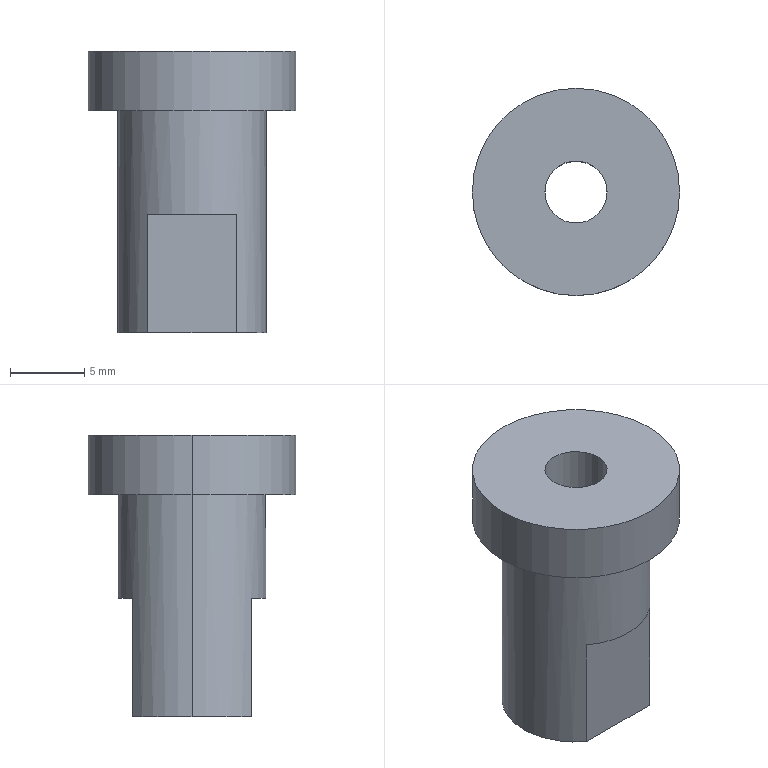Part | STEP file | PN_0015 Mount electronic clip cylinder connecting head | 1 solid | 13 faces | box 14 x 14 x 19 mm | volume 1465 mm3 | plane 7 | cylinder 6 | commonest cylinder face diameters 4.2 x2 10 x2 14 x2
STEP:
#1=CARTESIAN_POINT('',(0.,0.,0.));
#2=DIRECTION('',(0.,0.,1.));
#3=DIRECTION('',(1.,0.,0.));
#4=AXIS2_PLACEMENT_3D('',#1,#2,#3);
#5=CARTESIAN_POINT('',(-2.1,0.,19.));
#6=VERTEX_POINT('',#5);
#7=CARTESIAN_POINT('',(-2.1,0.,0.));
#8=VERTEX_POINT('',#7);
#9=CARTESIAN_POINT('',(-2.1,0.,0.));
#10=DIRECTION('',(0.,0.,-1.));
#11=VECTOR('',#10,1.);
#12=LINE('',#9,#11);
#13=CARTESIAN_POINT('',(0.,0.,0.));
#14=DIRECTION('',(0.,0.,-1.));
#15=DIRECTION('',(-1.,0.,0.));
#16=AXIS2_PLACEMENT_3D('',#13,#14,#15);
#17=CYLINDRICAL_SURFACE('',#16,2.1);
#18=CARTESIAN_POINT('',(6.283,0.));
#19=DIRECTION('',(0.,1.));
#20=VECTOR('',#19,1.);
#21=LINE('',#18,#20);
#22=(GEOMETRIC_REPRESENTATION_CONTEXT(2)PARAMETRIC_REPRESENTATION_CONTEXT()REPRESENTATION_CONTEXT('',''));
#23=DEFINITIONAL_REPRESENTATION('',(#21),#22);
#24=PCURVE('',#17,#23);
#25=CARTESIAN_POINT('',(0.,0.,0.));
#26=DIRECTION('',(0.,0.,-1.));
#27=DIRECTION('',(-1.,0.,0.));
#28=AXIS2_PLACEMENT_3D('',#25,#26,#27);
#29=CYLINDRICAL_SURFACE('',#28,2.1);
#30=CARTESIAN_POINT('',(0.,0.));
#31=DIRECTION('',(0.,1.));
#32=VECTOR('',#31,1.);
#33=LINE('',#30,#32);
#34=(GEOMETRIC_REPRESENTATION_CONTEXT(2)PARAMETRIC_REPRESENTATION_CONTEXT()REPRESENTATION_CONTEXT('',''));
#35=DEFINITIONAL_REPRESENTATION('',(#33),#34);
#36=PCURVE('',#29,#35);
#37=SURFACE_CURVE('',#12,(#24,#36),.PCURVE_S1.);
#38=EDGE_CURVE('',#6,#8,#37,.T.);
#39=ORIENTED_EDGE('',*,*,#38,.T.);
#40=CARTESIAN_POINT('',(2.1,0.,0.));
#41=VERTEX_POINT('',#40);
#42=CARTESIAN_POINT('',(0.,0.,0.));
#43=DIRECTION('',(0.,0.,-1.));
#44=DIRECTION('',(-1.,0.,0.));
#45=AXIS2_PLACEMENT_3D('',#42,#43,#44);
#46=CIRCLE('',#45,2.1);
#47=CARTESIAN_POINT('',(0.,0.));
#48=DIRECTION('',(1.,0.));
#49=VECTOR('',#48,1.);
#50=LINE('',#47,#49);
#51=(GEOMETRIC_REPRESENTATION_CONTEXT(2)PARAMETRIC_REPRESENTATION_CONTEXT()REPRESENTATION_CONTEXT('',''));
#52=DEFINITIONAL_REPRESENTATION('',(#50),#51);
#53=PCURVE('',#17,#52);
#54=CARTESIAN_POINT('',(0.,0.,0.));
#55=DIRECTION('',(0.,0.,1.));
#56=DIRECTION('',(1.,0.,0.));
#57=AXIS2_PLACEMENT_3D('',#54,#55,#56);
#58=PLANE('',#57);
#59=CARTESIAN_POINT('',(-2.1,0.));
#60=CARTESIAN_POINT('',(-2.1,3.637));
#61=CARTESIAN_POINT('',(1.05,1.819));
#62=CARTESIAN_POINT('',(4.2,0.));
#63=CARTESIAN_POINT('',(1.05,-1.819));
#64=CARTESIAN_POINT('',(-2.1,-3.637));
#65=CARTESIAN_POINT('',(-2.1,0.));
#66=(BOUNDED_CURVE()B_SPLINE_CURVE(2,(#59,#60,#61,#62,#63,#64,#65),.UNSPECIFIED.,.T.,.F.)B_SPLINE_CURVE_WITH_KNOTS((1,2,2,2,2,1),(-2.094,0.,2.094,4.189,6.283,8.378),.UNSPECIFIED.)CURVE()GEOMETRIC_REPRESENTATION_ITEM()RATIONAL_B_SPLINE_CURVE((1.,0.5,1.,0.5,1.,0.5,1.))REPRESENTATION_ITEM(''));
#67=(GEOMETRIC_REPRESENTATION_CONTEXT(2)PARAMETRIC_REPRESENTATION_CONTEXT()REPRESENTATION_CONTEXT('',''));
#68=DEFINITIONAL_REPRESENTATION('',(#66),#67);
#69=PCURVE('',#58,#68);
#70=SURFACE_CURVE('',#46,(#53,#69),.PCURVE_S1.);
#71=EDGE_CURVE('',#41,#8,#70,.T.);
#72=ORIENTED_EDGE('',*,*,#71,.F.);
#73=CARTESIAN_POINT('',(2.1,0.,19.));
#74=VERTEX_POINT('',#73);
#75=CARTESIAN_POINT('',(2.1,0.,0.));
#76=DIRECTION('',(0.,0.,-1.));
#77=VECTOR('',#76,1.);
#78=LINE('',#75,#77);
#79=CARTESIAN_POINT('',(3.142,0.));
#80=DIRECTION('',(0.,1.));
#81=VECTOR('',#80,1.);
#82=LINE('',#79,#81);
#83=(GEOMETRIC_REPRESENTATION_CONTEXT(2)PARAMETRIC_REPRESENTATION_CONTEXT()REPRESENTATION_CONTEXT('',''));
#84=DEFINITIONAL_REPRESENTATION('',(#82),#83);
#85=PCURVE('',#17,#84);
#86=CARTESIAN_POINT('',(3.142,0.));
#87=DIRECTION('',(0.,1.));
#88=VECTOR('',#87,1.);
#89=LINE('',#86,#88);
#90=(GEOMETRIC_REPRESENTATION_CONTEXT(2)PARAMETRIC_REPRESENTATION_CONTEXT()REPRESENTATION_CONTEXT('',''));
#91=DEFINITIONAL_REPRESENTATION('',(#89),#90);
#92=PCURVE('',#29,#91);
#93=SURFACE_CURVE('',#78,(#85,#92),.PCURVE_S1.);
#94=EDGE_CURVE('',#74,#41,#93,.T.);
#95=ORIENTED_EDGE('',*,*,#94,.F.);
#96=CARTESIAN_POINT('',(0.,0.,19.));
#97=DIRECTION('',(0.,0.,-1.));
#98=DIRECTION('',(-1.,0.,0.));
#99=AXIS2_PLACEMENT_3D('',#96,#97,#98);
#100=CIRCLE('',#99,2.1);
#101=CARTESIAN_POINT('',(0.,-19.));
#102=DIRECTION('',(1.,0.));
#103=VECTOR('',#102,1.);
#104=LINE('',#101,#103);
#105=(GEOMETRIC_REPRESENTATION_CONTEXT(2)PARAMETRIC_REPRESENTATION_CONTEXT()REPRESENTATION_CONTEXT('',''));
#106=DEFINITIONAL_REPRESENTATION('',(#104),#105);
#107=PCURVE('',#17,#106);
#108=CARTESIAN_POINT('',(0.,0.,19.));
#109=DIRECTION('',(0.,0.,1.));
#110=DIRECTION('',(1.,0.,0.));
#111=AXIS2_PLACEMENT_3D('',#108,#109,#110);
#112=PLANE('',#111);
#113=CARTESIAN_POINT('',(-2.1,0.));
#114=CARTESIAN_POINT('',(-2.1,3.637));
#115=CARTESIAN_POINT('',(1.05,1.819));
#116=CARTESIAN_POINT('',(4.2,0.));
#117=CARTESIAN_POINT('',(1.05,-1.819));
#118=CARTESIAN_POINT('',(-2.1,-3.637));
#119=CARTESIAN_POINT('',(-2.1,0.));
#120=(BOUNDED_CURVE()B_SPLINE_CURVE(2,(#113,#114,#115,#116,#117,#118,#119),.UNSPECIFIED.,.T.,.F.)B_SPLINE_CURVE_WITH_KNOTS((1,2,2,2,2,1),(-2.094,0.,2.094,4.189,6.283,8.378),.UNSPECIFIED.)CURVE()GEOMETRIC_REPRESENTATION_ITEM()RATIONAL_B_SPLINE_CURVE((1.,0.5,1.,0.5,1.,0.5,1.))REPRESENTATION_ITEM(''));
#121=(GEOMETRIC_REPRESENTATION_CONTEXT(2)PARAMETRIC_REPRESENTATION_CONTEXT()REPRESENTATION_CONTEXT('',''));
#122=DEFINITIONAL_REPRESENTATION('',(#120),#121);
#123=PCURVE('',#112,#122);
#124=SURFACE_CURVE('',#100,(#107,#123),.PCURVE_S1.);
#125=EDGE_CURVE('',#74,#6,#124,.T.);
#126=ORIENTED_EDGE('',*,*,#125,.T.);
#127=EDGE_LOOP('',(#39,#72,#95,#126));
#128=FACE_BOUND('',#127,.F.);
#129=ADVANCED_FACE('',(#128),#17,.F.);
#130=CARTESIAN_POINT('',(7.,0.,19.));
#131=VERTEX_POINT('',#130);
#132=CARTESIAN_POINT('',(-7.,0.,19.));
#133=VERTEX_POINT('',#132);
#134=CARTESIAN_POINT('',(0.,0.,19.));
#135=DIRECTION('',(0.,0.,1.));
#136=DIRECTION('',(1.,0.,0.));
#137=AXIS2_PLACEMENT_3D('',#134,#135,#136);
#138=CIRCLE('',#137,7.);
#139=CARTESIAN_POINT('',(0.,0.,19.));
#140=DIRECTION('',(0.,0.,-1.));
#141=DIRECTION('',(-1.,0.,0.));
#142=AXIS2_PLACEMENT_3D('',#139,#140,#141);
#143=CYLINDRICAL_SURFACE('',#142,7.);
#144=CARTESIAN_POINT('',(3.142,0.));
#145=DIRECTION('',(-1.,0.));
#146=VECTOR('',#145,1.);
#147=LINE('',#144,#146);
#148=(GEOMETRIC_REPRESENTATION_CONTEXT(2)PARAMETRIC_REPRESENTATION_CONTEXT()REPRESENTATION_CONTEXT('',''));
#149=DEFINITIONAL_REPRESENTATION('',(#147),#148);
#150=PCURVE('',#143,#149);
#151=CARTESIAN_POINT('',(0.,0.));
#152=DIRECTION('',(1.,0.));
#153=AXIS2_PLACEMENT_2D('',#151,#152);
#154=CIRCLE('',#153,7.);
#155=(GEOMETRIC_REPRESENTATION_CONTEXT(2)PARAMETRIC_REPRESENTATION_CONTEXT()REPRESENTATION_CONTEXT('',''));
#156=DEFINITIONAL_REPRESENTATION('',(#154),#155);
#157=PCURVE('',#112,#156);
#158=SURFACE_CURVE('',#138,(#150,#157),.PCURVE_S1.);
#159=EDGE_CURVE('',#131,#133,#158,.T.);
#160=ORIENTED_EDGE('',*,*,#159,.F.);
#161=CARTESIAN_POINT('',(7.,0.,15.));
#162=VERTEX_POINT('',#161);
#163=CARTESIAN_POINT('',(7.,0.,19.));
#164=DIRECTION('',(0.,0.,-1.));
#165=VECTOR('',#164,1.);
#166=LINE('',#163,#165);
#167=CARTESIAN_POINT('',(3.142,0.));
#168=DIRECTION('',(0.,1.));
#169=VECTOR('',#168,1.);
#170=LINE('',#167,#169);
#171=(GEOMETRIC_REPRESENTATION_CONTEXT(2)PARAMETRIC_REPRESENTATION_CONTEXT()REPRESENTATION_CONTEXT('',''));
#172=DEFINITIONAL_REPRESENTATION('',(#170),#171);
#173=PCURVE('',#143,#172);
#174=CARTESIAN_POINT('',(0.,0.,19.));
#175=DIRECTION('',(0.,0.,-1.));
#176=DIRECTION('',(-1.,0.,0.));
#177=AXIS2_PLACEMENT_3D('',#174,#175,#176);
#178=CYLINDRICAL_SURFACE('',#177,7.);
#179=CARTESIAN_POINT('',(3.142,0.));
#180=DIRECTION('',(0.,1.));
#181=VECTOR('',#180,1.);
#182=LINE('',#179,#181);
#183=(GEOMETRIC_REPRESENTATION_CONTEXT(2)PARAMETRIC_REPRESENTATION_CONTEXT()REPRESENTATION_CONTEXT('',''));
#184=DEFINITIONAL_REPRESENTATION('',(#182),#183);
#185=PCURVE('',#178,#184);
#186=SURFACE_CURVE('',#166,(#173,#185),.PCURVE_S1.);
#187=EDGE_CURVE('',#131,#162,#186,.T.);
#188=ORIENTED_EDGE('',*,*,#187,.T.);
#189=CARTESIAN_POINT('',(-7.,0.,15.));
#190=VERTEX_POINT('',#189);
#191=CARTESIAN_POINT('',(0.,0.,15.));
#192=DIRECTION('',(0.,0.,1.));
#193=DIRECTION('',(1.,0.,0.));
#194=AXIS2_PLACEMENT_3D('',#191,#192,#193);
#195=CIRCLE('',#194,7.);
#196=CARTESIAN_POINT('',(3.142,4.));
#197=DIRECTION('',(-1.,0.));
#198=VECTOR('',#197,1.);
#199=LINE('',#196,#198);
#200=(GEOMETRIC_REPRESENTATION_CONTEXT(2)PARAMETRIC_REPRESENTATION_CONTEXT()REPRESENTATION_CONTEXT('',''));
#201=DEFINITIONAL_REPRESENTATION('',(#199),#200);
#202=PCURVE('',#143,#201);
#203=CARTESIAN_POINT('',(0.,0.,15.));
#204=DIRECTION('',(0.,0.,1.));
#205=DIRECTION('',(1.,0.,0.));
#206=AXIS2_PLACEMENT_3D('',#203,#204,#205);
#207=PLANE('',#206);
#208=CARTESIAN_POINT('',(0.,0.));
#209=DIRECTION('',(1.,0.));
#210=AXIS2_PLACEMENT_2D('',#208,#209);
#211=CIRCLE('',#210,7.);
#212=(GEOMETRIC_REPRESENTATION_CONTEXT(2)PARAMETRIC_REPRESENTATION_CONTEXT()REPRESENTATION_CONTEXT('',''));
#213=DEFINITIONAL_REPRESENTATION('',(#211),#212);
#214=PCURVE('',#207,#213);
#215=SURFACE_CURVE('',#195,(#202,#214),.PCURVE_S1.);
#216=EDGE_CURVE('',#162,#190,#215,.T.);
#217=ORIENTED_EDGE('',*,*,#216,.T.);
#218=CARTESIAN_POINT('',(-7.,0.,19.));
#219=DIRECTION('',(0.,0.,-1.));
#220=VECTOR('',#219,1.);
#221=LINE('',#218,#220);
#222=CARTESIAN_POINT('',(0.,0.));
#223=DIRECTION('',(0.,1.));
#224=VECTOR('',#223,1.);
#225=LINE('',#222,#224);
#226=(GEOMETRIC_REPRESENTATION_CONTEXT(2)PARAMETRIC_REPRESENTATION_CONTEXT()REPRESENTATION_CONTEXT('',''));
#227=DEFINITIONAL_REPRESENTATION('',(#225),#226);
#228=PCURVE('',#143,#227);
#229=CARTESIAN_POINT('',(6.283,0.));
#230=DIRECTION('',(0.,1.));
#231=VECTOR('',#230,1.);
#232=LINE('',#229,#231);
#233=(GEOMETRIC_REPRESENTATION_CONTEXT(2)PARAMETRIC_REPRESENTATION_CONTEXT()REPRESENTATION_CONTEXT('',''));
#234=DEFINITIONAL_REPRESENTATION('',(#232),#233);
#235=PCURVE('',#178,#234);
#236=SURFACE_CURVE('',#221,(#228,#235),.PCURVE_S1.);
#237=EDGE_CURVE('',#133,#190,#236,.T.);
#238=ORIENTED_EDGE('',*,*,#237,.F.);
#239=EDGE_LOOP('',(#160,#188,#217,#238));
#240=FACE_BOUND('',#239,.T.);
#241=ADVANCED_FACE('',(#240),#143,.T.);
#242=CARTESIAN_POINT('',(5.,0.,15.));
#243=VERTEX_POINT('',#242);
#244=CARTESIAN_POINT('',(-5.,0.,15.));
#245=VERTEX_POINT('',#244);
#246=CARTESIAN_POINT('',(0.,0.,15.));
#247=DIRECTION('',(0.,0.,1.));
#248=DIRECTION('',(1.,0.,0.));
#249=AXIS2_PLACEMENT_3D('',#246,#247,#248);
#250=CIRCLE('',#249,5.);
#251=CARTESIAN_POINT('',(0.,0.,15.));
#252=DIRECTION('',(0.,0.,-1.));
#253=DIRECTION('',(-1.,0.,0.));
#254=AXIS2_PLACEMENT_3D('',#251,#252,#253);
#255=CYLINDRICAL_SURFACE('',#254,5.);
#256=CARTESIAN_POINT('',(3.142,0.));
#257=DIRECTION('',(-1.,0.));
#258=VECTOR('',#257,1.);
#259=LINE('',#256,#258);
#260=(GEOMETRIC_REPRESENTATION_CONTEXT(2)PARAMETRIC_REPRESENTATION_CONTEXT()REPRESENTATION_CONTEXT('',''));
#261=DEFINITIONAL_REPRESENTATION('',(#259),#260);
#262=PCURVE('',#255,#261);
#263=CARTESIAN_POINT('',(0.,0.));
#264=DIRECTION('',(1.,0.));
#265=AXIS2_PLACEMENT_2D('',#263,#264);
#266=CIRCLE('',#265,5.);
#267=(GEOMETRIC_REPRESENTATION_CONTEXT(2)PARAMETRIC_REPRESENTATION_CONTEXT()REPRESENTATION_CONTEXT('',''));
#268=DEFINITIONAL_REPRESENTATION('',(#266),#267);
#269=PCURVE('',#207,#268);
#270=SURFACE_CURVE('',#250,(#262,#269),.PCURVE_S1.);
#271=EDGE_CURVE('',#243,#245,#270,.T.);
#272=ORIENTED_EDGE('',*,*,#271,.F.);
#273=CARTESIAN_POINT('',(5.,0.,0.));
#274=VERTEX_POINT('',#273);
#275=CARTESIAN_POINT('',(5.,0.,15.));
#276=DIRECTION('',(0.,0.,-1.));
#277=VECTOR('',#276,1.);
#278=LINE('',#275,#277);
#279=CARTESIAN_POINT('',(3.142,0.));
#280=DIRECTION('',(0.,1.));
#281=VECTOR('',#280,1.);
#282=LINE('',#279,#281);
#283=(GEOMETRIC_REPRESENTATION_CONTEXT(2)PARAMETRIC_REPRESENTATION_CONTEXT()REPRESENTATION_CONTEXT('',''));
#284=DEFINITIONAL_REPRESENTATION('',(#282),#283);
#285=PCURVE('',#255,#284);
#286=CARTESIAN_POINT('',(0.,0.,15.));
#287=DIRECTION('',(0.,0.,-1.));
#288=DIRECTION('',(-1.,0.,0.));
#289=AXIS2_PLACEMENT_3D('',#286,#287,#288);
#290=CYLINDRICAL_SURFACE('',#289,5.);
#291=CARTESIAN_POINT('',(3.142,0.));
#292=DIRECTION('',(0.,1.));
#293=VECTOR('',#292,1.);
#294=LINE('',#291,#293);
#295=(GEOMETRIC_REPRESENTATION_CONTEXT(2)PARAMETRIC_REPRESENTATION_CONTEXT()REPRESENTATION_CONTEXT('',''));
#296=DEFINITIONAL_REPRESENTATION('',(#294),#295);
#297=PCURVE('',#290,#296);
#298=SURFACE_CURVE('',#278,(#285,#297),.PCURVE_S1.);
#299=EDGE_CURVE('',#243,#274,#298,.T.);
#300=ORIENTED_EDGE('',*,*,#299,.T.);
#301=CARTESIAN_POINT('',(3.,4.,0.));
#302=VERTEX_POINT('',#301);
#303=CARTESIAN_POINT('',(0.,0.,0.));
#304=DIRECTION('',(0.,0.,1.));
#305=DIRECTION('',(1.,0.,0.));
#306=AXIS2_PLACEMENT_3D('',#303,#304,#305);
#307=CIRCLE('',#306,5.);
#308=CARTESIAN_POINT('',(3.142,15.));
#309=DIRECTION('',(-1.,0.));
#310=VECTOR('',#309,1.);
#311=LINE('',#308,#310);
#312=(GEOMETRIC_REPRESENTATION_CONTEXT(2)PARAMETRIC_REPRESENTATION_CONTEXT()REPRESENTATION_CONTEXT('',''));
#313=DEFINITIONAL_REPRESENTATION('',(#311),#312);
#314=PCURVE('',#255,#313);
#315=CARTESIAN_POINT('',(0.,0.));
#316=DIRECTION('',(1.,0.));
#317=AXIS2_PLACEMENT_2D('',#315,#316);
#318=CIRCLE('',#317,5.);
#319=(GEOMETRIC_REPRESENTATION_CONTEXT(2)PARAMETRIC_REPRESENTATION_CONTEXT()REPRESENTATION_CONTEXT('',''));
#320=DEFINITIONAL_REPRESENTATION('',(#318),#319);
#321=PCURVE('',#58,#320);
#322=SURFACE_CURVE('',#307,(#314,#321),.PCURVE_S1.);
#323=EDGE_CURVE('',#274,#302,#322,.T.);
#324=ORIENTED_EDGE('',*,*,#323,.T.);
#325=CARTESIAN_POINT('',(3.,4.,8.));
#326=VERTEX_POINT('',#325);
#327=CARTESIAN_POINT('',(3.,4.,15.));
#328=DIRECTION('',(0.,0.,1.));
#329=VECTOR('',#328,1.);
#330=LINE('',#327,#329);
#331=CARTESIAN_POINT('',(2.214,0.));
#332=DIRECTION('',(0.,-1.));
#333=VECTOR('',#332,1.);
#334=LINE('',#331,#333);
#335=(GEOMETRIC_REPRESENTATION_CONTEXT(2)PARAMETRIC_REPRESENTATION_CONTEXT()REPRESENTATION_CONTEXT('',''));
#336=DEFINITIONAL_REPRESENTATION('',(#334),#335);
#337=PCURVE('',#255,#336);
#338=CARTESIAN_POINT('',(5.893,4.,8.));
#339=DIRECTION('',(0.,-1.,0.));
#340=DIRECTION('',(1.,0.,0.));
#341=AXIS2_PLACEMENT_3D('',#338,#339,#340);
#342=PLANE('',#341);
#343=CARTESIAN_POINT('',(-2.893,7.));
#344=DIRECTION('',(0.,1.));
#345=VECTOR('',#344,1.);
#346=LINE('',#343,#345);
#347=(GEOMETRIC_REPRESENTATION_CONTEXT(2)PARAMETRIC_REPRESENTATION_CONTEXT()REPRESENTATION_CONTEXT('',''));
#348=DEFINITIONAL_REPRESENTATION('',(#346),#347);
#349=PCURVE('',#342,#348);
#350=SURFACE_CURVE('',#330,(#337,#349),.PCURVE_S1.);
#351=EDGE_CURVE('',#302,#326,#350,.T.);
#352=ORIENTED_EDGE('',*,*,#351,.T.);
#353=CARTESIAN_POINT('',(-3.,4.,8.));
#354=VERTEX_POINT('',#353);
#355=CARTESIAN_POINT('',(0.,0.,8.));
#356=DIRECTION('',(0.,0.,-1.));
#357=DIRECTION('',(-1.,0.,0.));
#358=AXIS2_PLACEMENT_3D('',#355,#356,#357);
#359=CIRCLE('',#358,5.);
#360=CARTESIAN_POINT('',(0.,7.));
#361=DIRECTION('',(1.,0.));
#362=VECTOR('',#361,1.);
#363=LINE('',#360,#362);
#364=(GEOMETRIC_REPRESENTATION_CONTEXT(2)PARAMETRIC_REPRESENTATION_CONTEXT()REPRESENTATION_CONTEXT('',''));
#365=DEFINITIONAL_REPRESENTATION('',(#363),#364);
#366=PCURVE('',#255,#365);
#367=CARTESIAN_POINT('',(0.,0.,8.));
#368=DIRECTION('',(0.,0.,-1.));
#369=DIRECTION('',(-1.,0.,0.));
#370=AXIS2_PLACEMENT_3D('',#367,#368,#369);
#371=PLANE('',#370);
#372=CARTESIAN_POINT('',(0.,0.));
#373=DIRECTION('',(1.,0.));
#374=AXIS2_PLACEMENT_2D('',#372,#373);
#375=CIRCLE('',#374,5.);
#376=(GEOMETRIC_REPRESENTATION_CONTEXT(2)PARAMETRIC_REPRESENTATION_CONTEXT()REPRESENTATION_CONTEXT('',''));
#377=DEFINITIONAL_REPRESENTATION('',(#375),#376);
#378=PCURVE('',#371,#377);
#379=SURFACE_CURVE('',#359,(#366,#378),.PCURVE_S1.);
#380=EDGE_CURVE('',#354,#326,#379,.T.);
#381=ORIENTED_EDGE('',*,*,#380,.F.);
#382=CARTESIAN_POINT('',(-3.,4.,0.));
#383=VERTEX_POINT('',#382);
#384=CARTESIAN_POINT('',(-3.,4.,15.));
#385=DIRECTION('',(0.,0.,-1.));
#386=VECTOR('',#385,1.);
#387=LINE('',#384,#386);
#388=CARTESIAN_POINT('',(0.9273,0.));
#389=DIRECTION('',(0.,1.));
#390=VECTOR('',#389,1.);
#391=LINE('',#388,#390);
#392=(GEOMETRIC_REPRESENTATION_CONTEXT(2)PARAMETRIC_REPRESENTATION_CONTEXT()REPRESENTATION_CONTEXT('',''));
#393=DEFINITIONAL_REPRESENTATION('',(#391),#392);
#394=PCURVE('',#255,#393);
#395=CARTESIAN_POINT('',(-8.893,7.));
#396=DIRECTION('',(0.,-1.));
#397=VECTOR('',#396,1.);
#398=LINE('',#395,#397);
#399=(GEOMETRIC_REPRESENTATION_CONTEXT(2)PARAMETRIC_REPRESENTATION_CONTEXT()REPRESENTATION_CONTEXT('',''));
#400=DEFINITIONAL_REPRESENTATION('',(#398),#399);
#401=PCURVE('',#342,#400);
#402=SURFACE_CURVE('',#387,(#394,#401),.PCURVE_S1.);
#403=EDGE_CURVE('',#354,#383,#402,.T.);
#404=ORIENTED_EDGE('',*,*,#403,.T.);
#405=CARTESIAN_POINT('',(-5.,0.,0.));
#406=VERTEX_POINT('',#405);
#407=CARTESIAN_POINT('',(0.,0.,0.));
#408=DIRECTION('',(0.,0.,1.));
#409=DIRECTION('',(1.,0.,0.));
#410=AXIS2_PLACEMENT_3D('',#407,#408,#409);
#411=CIRCLE('',#410,5.);
#412=CARTESIAN_POINT('',(3.142,15.));
#413=DIRECTION('',(-1.,0.));
#414=VECTOR('',#413,1.);
#415=LINE('',#412,#414);
#416=(GEOMETRIC_REPRESENTATION_CONTEXT(2)PARAMETRIC_REPRESENTATION_CONTEXT()REPRESENTATION_CONTEXT('',''));
#417=DEFINITIONAL_REPRESENTATION('',(#415),#416);
#418=PCURVE('',#255,#417);
#419=CARTESIAN_POINT('',(0.,0.));
#420=DIRECTION('',(1.,0.));
#421=AXIS2_PLACEMENT_2D('',#419,#420);
#422=CIRCLE('',#421,5.);
#423=(GEOMETRIC_REPRESENTATION_CONTEXT(2)PARAMETRIC_REPRESENTATION_CONTEXT()REPRESENTATION_CONTEXT('',''));
#424=DEFINITIONAL_REPRESENTATION('',(#422),#423);
#425=PCURVE('',#58,#424);
#426=SURFACE_CURVE('',#411,(#418,#425),.PCURVE_S1.);
#427=EDGE_CURVE('',#383,#406,#426,.T.);
#428=ORIENTED_EDGE('',*,*,#427,.T.);
#429=CARTESIAN_POINT('',(-5.,0.,15.));
#430=DIRECTION('',(0.,0.,-1.));
#431=VECTOR('',#430,1.);
#432=LINE('',#429,#431);
#433=CARTESIAN_POINT('',(0.,0.));
#434=DIRECTION('',(0.,1.));
#435=VECTOR('',#434,1.);
#436=LINE('',#433,#435);
#437=(GEOMETRIC_REPRESENTATION_CONTEXT(2)PARAMETRIC_REPRESENTATION_CONTEXT()REPRESENTATION_CONTEXT('',''));
#438=DEFINITIONAL_REPRESENTATION('',(#436),#437);
#439=PCURVE('',#255,#438);
#440=CARTESIAN_POINT('',(6.283,0.));
#441=DIRECTION('',(0.,1.));
#442=VECTOR('',#441,1.);
#443=LINE('',#440,#442);
#444=(GEOMETRIC_REPRESENTATION_CONTEXT(2)PARAMETRIC_REPRESENTATION_CONTEXT()REPRESENTATION_CONTEXT('',''));
#445=DEFINITIONAL_REPRESENTATION('',(#443),#444);
#446=PCURVE('',#290,#445);
#447=SURFACE_CURVE('',#432,(#439,#446),.PCURVE_S1.);
#448=EDGE_CURVE('',#245,#406,#447,.T.);
#449=ORIENTED_EDGE('',*,*,#448,.F.);
#450=EDGE_LOOP('',(#272,#300,#324,#352,#381,#404,#428,#449));
#451=FACE_BOUND('',#450,.T.);
#452=ADVANCED_FACE('',(#451),#255,.T.);
#453=CARTESIAN_POINT('',(0.,0.,19.));
#454=DIRECTION('',(0.,0.,1.));
#455=DIRECTION('',(1.,0.,0.));
#456=AXIS2_PLACEMENT_3D('',#453,#454,#455);
#457=CIRCLE('',#456,7.);
#458=CARTESIAN_POINT('',(0.,0.));
#459=DIRECTION('',(1.,0.));
#460=AXIS2_PLACEMENT_2D('',#458,#459);
#461=CIRCLE('',#460,7.);
#462=(GEOMETRIC_REPRESENTATION_CONTEXT(2)PARAMETRIC_REPRESENTATION_CONTEXT()REPRESENTATION_CONTEXT('',''));
#463=DEFINITIONAL_REPRESENTATION('',(#461),#462);
#464=PCURVE('',#112,#463);
#465=CARTESIAN_POINT('',(9.425,0.));
#466=DIRECTION('',(-1.,0.));
#467=VECTOR('',#466,1.);
#468=LINE('',#465,#467);
#469=(GEOMETRIC_REPRESENTATION_CONTEXT(2)PARAMETRIC_REPRESENTATION_CONTEXT()REPRESENTATION_CONTEXT('',''));
#470=DEFINITIONAL_REPRESENTATION('',(#468),#469);
#471=PCURVE('',#178,#470);
#472=SURFACE_CURVE('',#457,(#464,#471),.PCURVE_S1.);
#473=EDGE_CURVE('',#133,#131,#472,.T.);
#474=ORIENTED_EDGE('',*,*,#473,.T.);
#475=ORIENTED_EDGE('',*,*,#159,.T.);
#476=EDGE_LOOP('',(#474,#475));
#477=FACE_BOUND('',#476,.T.);
#478=CARTESIAN_POINT('',(0.,0.,19.));
#479=DIRECTION('',(0.,0.,-1.));
#480=DIRECTION('',(-1.,0.,0.));
#481=AXIS2_PLACEMENT_3D('',#478,#479,#480);
#482=CIRCLE('',#481,2.1);
#483=CARTESIAN_POINT('',(-2.1,0.));
#484=CARTESIAN_POINT('',(-2.1,3.637));
#485=CARTESIAN_POINT('',(1.05,1.819));
#486=CARTESIAN_POINT('',(4.2,0.));
#487=CARTESIAN_POINT('',(1.05,-1.819));
#488=CARTESIAN_POINT('',(-2.1,-3.637));
#489=CARTESIAN_POINT('',(-2.1,0.));
#490=(BOUNDED_CURVE()B_SPLINE_CURVE(2,(#483,#484,#485,#486,#487,#488,#489),.UNSPECIFIED.,.T.,.F.)B_SPLINE_CURVE_WITH_KNOTS((1,2,2,2,2,1),(-2.094,0.,2.094,4.189,6.283,8.378),.UNSPECIFIED.)CURVE()GEOMETRIC_REPRESENTATION_ITEM()RATIONAL_B_SPLINE_CURVE((1.,0.5,1.,0.5,1.,0.5,1.))REPRESENTATION_ITEM(''));
#491=(GEOMETRIC_REPRESENTATION_CONTEXT(2)PARAMETRIC_REPRESENTATION_CONTEXT()REPRESENTATION_CONTEXT('',''));
#492=DEFINITIONAL_REPRESENTATION('',(#490),#491);
#493=PCURVE('',#112,#492);
#494=CARTESIAN_POINT('',(0.,-19.));
#495=DIRECTION('',(1.,0.));
#496=VECTOR('',#495,1.);
#497=LINE('',#494,#496);
#498=(GEOMETRIC_REPRESENTATION_CONTEXT(2)PARAMETRIC_REPRESENTATION_CONTEXT()REPRESENTATION_CONTEXT('',''));
#499=DEFINITIONAL_REPRESENTATION('',(#497),#498);
#500=PCURVE('',#29,#499);
#501=SURFACE_CURVE('',#482,(#493,#500),.PCURVE_S1.);
#502=EDGE_CURVE('',#6,#74,#501,.T.);
#503=ORIENTED_EDGE('',*,*,#502,.T.);
#504=ORIENTED_EDGE('',*,*,#125,.T.);
#505=EDGE_LOOP('',(#503,#504));
#506=FACE_BOUND('',#505,.T.);
#507=ADVANCED_FACE('',(#477,#506),#112,.T.);
#508=ORIENTED_EDGE('',*,*,#299,.F.);
#509=CARTESIAN_POINT('',(0.,0.,15.));
#510=DIRECTION('',(0.,0.,1.));
#511=DIRECTION('',(1.,0.,0.));
#512=AXIS2_PLACEMENT_3D('',#509,#510,#511);
#513=CIRCLE('',#512,5.);
#514=CARTESIAN_POINT('',(9.425,0.));
#515=DIRECTION('',(-1.,0.));
#516=VECTOR('',#515,1.);
#517=LINE('',#514,#516);
#518=(GEOMETRIC_REPRESENTATION_CONTEXT(2)PARAMETRIC_REPRESENTATION_CONTEXT()REPRESENTATION_CONTEXT('',''));
#519=DEFINITIONAL_REPRESENTATION('',(#517),#518);
#520=PCURVE('',#290,#519);
#521=CARTESIAN_POINT('',(0.,0.));
#522=DIRECTION('',(1.,0.));
#523=AXIS2_PLACEMENT_2D('',#521,#522);
#524=CIRCLE('',#523,5.);
#525=(GEOMETRIC_REPRESENTATION_CONTEXT(2)PARAMETRIC_REPRESENTATION_CONTEXT()REPRESENTATION_CONTEXT('',''));
#526=DEFINITIONAL_REPRESENTATION('',(#524),#525);
#527=PCURVE('',#207,#526);
#528=SURFACE_CURVE('',#513,(#520,#527),.PCURVE_S1.);
#529=EDGE_CURVE('',#245,#243,#528,.T.);
#530=ORIENTED_EDGE('',*,*,#529,.F.);
#531=ORIENTED_EDGE('',*,*,#448,.T.);
#532=CARTESIAN_POINT('',(-3.,-4.,0.));
#533=VERTEX_POINT('',#532);
#534=CARTESIAN_POINT('',(0.,0.,0.));
#535=DIRECTION('',(0.,0.,1.));
#536=DIRECTION('',(1.,0.,0.));
#537=AXIS2_PLACEMENT_3D('',#534,#535,#536);
#538=CIRCLE('',#537,5.);
#539=CARTESIAN_POINT('',(9.425,15.));
#540=DIRECTION('',(-1.,0.));
#541=VECTOR('',#540,1.);
#542=LINE('',#539,#541);
#543=(GEOMETRIC_REPRESENTATION_CONTEXT(2)PARAMETRIC_REPRESENTATION_CONTEXT()REPRESENTATION_CONTEXT('',''));
#544=DEFINITIONAL_REPRESENTATION('',(#542),#543);
#545=PCURVE('',#290,#544);
#546=CARTESIAN_POINT('',(0.,0.));
#547=DIRECTION('',(1.,0.));
#548=AXIS2_PLACEMENT_2D('',#546,#547);
#549=CIRCLE('',#548,5.);
#550=(GEOMETRIC_REPRESENTATION_CONTEXT(2)PARAMETRIC_REPRESENTATION_CONTEXT()REPRESENTATION_CONTEXT('',''));
#551=DEFINITIONAL_REPRESENTATION('',(#549),#550);
#552=PCURVE('',#58,#551);
#553=SURFACE_CURVE('',#538,(#545,#552),.PCURVE_S1.);
#554=EDGE_CURVE('',#406,#533,#553,.T.);
#555=ORIENTED_EDGE('',*,*,#554,.T.);
#556=CARTESIAN_POINT('',(-3.,-4.,8.));
#557=VERTEX_POINT('',#556);
#558=CARTESIAN_POINT('',(-3.,-4.,15.));
#559=DIRECTION('',(0.,0.,1.));
#560=VECTOR('',#559,1.);
#561=LINE('',#558,#560);
#562=CARTESIAN_POINT('',(5.356,0.));
#563=DIRECTION('',(0.,-1.));
#564=VECTOR('',#563,1.);
#565=LINE('',#562,#564);
#566=(GEOMETRIC_REPRESENTATION_CONTEXT(2)PARAMETRIC_REPRESENTATION_CONTEXT()REPRESENTATION_CONTEXT('',''));
#567=DEFINITIONAL_REPRESENTATION('',(#565),#566);
#568=PCURVE('',#290,#567);
#569=CARTESIAN_POINT('',(-8.893,-4.,8.));
#570=DIRECTION('',(0.,1.,0.));
#571=DIRECTION('',(-1.,0.,0.));
#572=AXIS2_PLACEMENT_3D('',#569,#570,#571);
#573=PLANE('',#572);
#574=CARTESIAN_POINT('',(-5.893,7.));
#575=DIRECTION('',(0.,1.));
#576=VECTOR('',#575,1.);
#577=LINE('',#574,#576);
#578=(GEOMETRIC_REPRESENTATION_CONTEXT(2)PARAMETRIC_REPRESENTATION_CONTEXT()REPRESENTATION_CONTEXT('',''));
#579=DEFINITIONAL_REPRESENTATION('',(#577),#578);
#580=PCURVE('',#573,#579);
#581=SURFACE_CURVE('',#561,(#568,#580),.PCURVE_S1.);
#582=EDGE_CURVE('',#533,#557,#581,.T.);
#583=ORIENTED_EDGE('',*,*,#582,.T.);
#584=CARTESIAN_POINT('',(3.,-4.,8.));
#585=VERTEX_POINT('',#584);
#586=CARTESIAN_POINT('',(0.,0.,8.));
#587=DIRECTION('',(0.,0.,-1.));
#588=DIRECTION('',(-1.,0.,0.));
#589=AXIS2_PLACEMENT_3D('',#586,#587,#588);
#590=CIRCLE('',#589,5.);
#591=CARTESIAN_POINT('',(0.,7.));
#592=DIRECTION('',(1.,0.));
#593=VECTOR('',#592,1.);
#594=LINE('',#591,#593);
#595=(GEOMETRIC_REPRESENTATION_CONTEXT(2)PARAMETRIC_REPRESENTATION_CONTEXT()REPRESENTATION_CONTEXT('',''));
#596=DEFINITIONAL_REPRESENTATION('',(#594),#595);
#597=PCURVE('',#290,#596);
#598=CARTESIAN_POINT('',(0.,0.,8.));
#599=DIRECTION('',(0.,0.,-1.));
#600=DIRECTION('',(-1.,0.,0.));
#601=AXIS2_PLACEMENT_3D('',#598,#599,#600);
#602=PLANE('',#601);
#603=CARTESIAN_POINT('',(0.,0.));
#604=DIRECTION('',(1.,0.));
#605=AXIS2_PLACEMENT_2D('',#603,#604);
#606=CIRCLE('',#605,5.);
#607=(GEOMETRIC_REPRESENTATION_CONTEXT(2)PARAMETRIC_REPRESENTATION_CONTEXT()REPRESENTATION_CONTEXT('',''));
#608=DEFINITIONAL_REPRESENTATION('',(#606),#607);
#609=PCURVE('',#602,#608);
#610=SURFACE_CURVE('',#590,(#597,#609),.PCURVE_S1.);
#611=EDGE_CURVE('',#585,#557,#610,.T.);
#612=ORIENTED_EDGE('',*,*,#611,.F.);
#613=CARTESIAN_POINT('',(3.,-4.,0.));
#614=VERTEX_POINT('',#613);
#615=CARTESIAN_POINT('',(3.,-4.,15.));
#616=DIRECTION('',(0.,0.,-1.));
#617=VECTOR('',#616,1.);
#618=LINE('',#615,#617);
#619=CARTESIAN_POINT('',(4.069,0.));
#620=DIRECTION('',(0.,1.));
#621=VECTOR('',#620,1.);
#622=LINE('',#619,#621);
#623=(GEOMETRIC_REPRESENTATION_CONTEXT(2)PARAMETRIC_REPRESENTATION_CONTEXT()REPRESENTATION_CONTEXT('',''));
#624=DEFINITIONAL_REPRESENTATION('',(#622),#623);
#625=PCURVE('',#290,#624);
#626=CARTESIAN_POINT('',(-11.893,7.));
#627=DIRECTION('',(0.,-1.));
#628=VECTOR('',#627,1.);
#629=LINE('',#626,#628);
#630=(GEOMETRIC_REPRESENTATION_CONTEXT(2)PARAMETRIC_REPRESENTATION_CONTEXT()REPRESENTATION_CONTEXT('',''));
#631=DEFINITIONAL_REPRESENTATION('',(#629),#630);
#632=PCURVE('',#573,#631);
#633=SURFACE_CURVE('',#618,(#625,#632),.PCURVE_S1.);
#634=EDGE_CURVE('',#585,#614,#633,.T.);
#635=ORIENTED_EDGE('',*,*,#634,.T.);
#636=CARTESIAN_POINT('',(0.,0.,0.));
#637=DIRECTION('',(0.,0.,1.));
#638=DIRECTION('',(1.,0.,0.));
#639=AXIS2_PLACEMENT_3D('',#636,#637,#638);
#640=CIRCLE('',#639,5.);
#641=CARTESIAN_POINT('',(9.425,15.));
#642=DIRECTION('',(-1.,0.));
#643=VECTOR('',#642,1.);
#644=LINE('',#641,#643);
#645=(GEOMETRIC_REPRESENTATION_CONTEXT(2)PARAMETRIC_REPRESENTATION_CONTEXT()REPRESENTATION_CONTEXT('',''));
#646=DEFINITIONAL_REPRESENTATION('',(#644),#645);
#647=PCURVE('',#290,#646);
#648=CARTESIAN_POINT('',(0.,0.));
#649=DIRECTION('',(1.,0.));
#650=AXIS2_PLACEMENT_2D('',#648,#649);
#651=CIRCLE('',#650,5.);
#652=(GEOMETRIC_REPRESENTATION_CONTEXT(2)PARAMETRIC_REPRESENTATION_CONTEXT()REPRESENTATION_CONTEXT('',''));
#653=DEFINITIONAL_REPRESENTATION('',(#651),#652);
#654=PCURVE('',#58,#653);
#655=SURFACE_CURVE('',#640,(#647,#654),.PCURVE_S1.);
#656=EDGE_CURVE('',#614,#274,#655,.T.);
#657=ORIENTED_EDGE('',*,*,#656,.T.);
#658=EDGE_LOOP('',(#508,#530,#531,#555,#583,#612,#635,#657));
#659=FACE_BOUND('',#658,.T.);
#660=ADVANCED_FACE('',(#659),#290,.T.);
#661=CARTESIAN_POINT('',(0.,0.,0.));
#662=DIRECTION('',(0.,0.,-1.));
#663=DIRECTION('',(-1.,0.,0.));
#664=AXIS2_PLACEMENT_3D('',#661,#662,#663);
#665=CIRCLE('',#664,2.1);
#666=CARTESIAN_POINT('',(-2.1,0.));
#667=CARTESIAN_POINT('',(-2.1,3.637));
#668=CARTESIAN_POINT('',(1.05,1.819));
#669=CARTESIAN_POINT('',(4.2,0.));
#670=CARTESIAN_POINT('',(1.05,-1.819));
#671=CARTESIAN_POINT('',(-2.1,-3.637));
#672=CARTESIAN_POINT('',(-2.1,0.));
#673=(BOUNDED_CURVE()B_SPLINE_CURVE(2,(#666,#667,#668,#669,#670,#671,#672),.UNSPECIFIED.,.T.,.F.)B_SPLINE_CURVE_WITH_KNOTS((1,2,2,2,2,1),(-2.094,0.,2.094,4.189,6.283,8.378),.UNSPECIFIED.)CURVE()GEOMETRIC_REPRESENTATION_ITEM()RATIONAL_B_SPLINE_CURVE((1.,0.5,1.,0.5,1.,0.5,1.))REPRESENTATION_ITEM(''));
#674=(GEOMETRIC_REPRESENTATION_CONTEXT(2)PARAMETRIC_REPRESENTATION_CONTEXT()REPRESENTATION_CONTEXT('',''));
#675=DEFINITIONAL_REPRESENTATION('',(#673),#674);
#676=PCURVE('',#58,#675);
#677=CARTESIAN_POINT('',(0.,0.));
#678=DIRECTION('',(1.,0.));
#679=VECTOR('',#678,1.);
#680=LINE('',#677,#679);
#681=(GEOMETRIC_REPRESENTATION_CONTEXT(2)PARAMETRIC_REPRESENTATION_CONTEXT()REPRESENTATION_CONTEXT('',''));
#682=DEFINITIONAL_REPRESENTATION('',(#680),#681);
#683=PCURVE('',#29,#682);
#684=SURFACE_CURVE('',#665,(#676,#683),.PCURVE_S1.);
#685=EDGE_CURVE('',#8,#41,#684,.T.);
#686=ORIENTED_EDGE('',*,*,#685,.F.);
#687=ORIENTED_EDGE('',*,*,#71,.F.);
#688=EDGE_LOOP('',(#686,#687));
#689=FACE_BOUND('',#688,.T.);
#690=ORIENTED_EDGE('',*,*,#656,.F.);
#691=CARTESIAN_POINT('',(0.,-4.,0.));
#692=DIRECTION('',(-1.,0.,0.));
#693=VECTOR('',#692,1.);
#694=LINE('',#691,#693);
#695=CARTESIAN_POINT('',(0.,-4.));
#696=DIRECTION('',(-1.,0.));
#697=VECTOR('',#696,1.);
#698=LINE('',#695,#697);
#699=(GEOMETRIC_REPRESENTATION_CONTEXT(2)PARAMETRIC_REPRESENTATION_CONTEXT()REPRESENTATION_CONTEXT('',''));
#700=DEFINITIONAL_REPRESENTATION('',(#698),#699);
#701=PCURVE('',#58,#700);
#702=CARTESIAN_POINT('',(-8.893,-8.));
#703=DIRECTION('',(1.,0.));
#704=VECTOR('',#703,1.);
#705=LINE('',#702,#704);
#706=(GEOMETRIC_REPRESENTATION_CONTEXT(2)PARAMETRIC_REPRESENTATION_CONTEXT()REPRESENTATION_CONTEXT('',''));
#707=DEFINITIONAL_REPRESENTATION('',(#705),#706);
#708=PCURVE('',#573,#707);
#709=SURFACE_CURVE('',#694,(#701,#708),.PCURVE_S1.);
#710=EDGE_CURVE('',#614,#533,#709,.T.);
#711=ORIENTED_EDGE('',*,*,#710,.T.);
#712=ORIENTED_EDGE('',*,*,#554,.F.);
#713=ORIENTED_EDGE('',*,*,#427,.F.);
#714=CARTESIAN_POINT('',(0.,4.,0.));
#715=DIRECTION('',(1.,0.,0.));
#716=VECTOR('',#715,1.);
#717=LINE('',#714,#716);
#718=CARTESIAN_POINT('',(0.,4.));
#719=DIRECTION('',(1.,0.));
#720=VECTOR('',#719,1.);
#721=LINE('',#718,#720);
#722=(GEOMETRIC_REPRESENTATION_CONTEXT(2)PARAMETRIC_REPRESENTATION_CONTEXT()REPRESENTATION_CONTEXT('',''));
#723=DEFINITIONAL_REPRESENTATION('',(#721),#722);
#724=PCURVE('',#58,#723);
#725=CARTESIAN_POINT('',(-5.893,-8.));
#726=DIRECTION('',(1.,0.));
#727=VECTOR('',#726,1.);
#728=LINE('',#725,#727);
#729=(GEOMETRIC_REPRESENTATION_CONTEXT(2)PARAMETRIC_REPRESENTATION_CONTEXT()REPRESENTATION_CONTEXT('',''));
#730=DEFINITIONAL_REPRESENTATION('',(#728),#729);
#731=PCURVE('',#342,#730);
#732=SURFACE_CURVE('',#717,(#724,#731),.PCURVE_S1.);
#733=EDGE_CURVE('',#383,#302,#732,.T.);
#734=ORIENTED_EDGE('',*,*,#733,.T.);
#735=ORIENTED_EDGE('',*,*,#323,.F.);
#736=EDGE_LOOP('',(#690,#711,#712,#713,#734,#735));
#737=FACE_BOUND('',#736,.T.);
#738=ADVANCED_FACE('',(#689,#737),#58,.F.);
#739=CARTESIAN_POINT('',(0.,0.,15.));
#740=DIRECTION('',(0.,0.,1.));
#741=DIRECTION('',(1.,0.,0.));
#742=AXIS2_PLACEMENT_3D('',#739,#740,#741);
#743=CIRCLE('',#742,7.);
#744=CARTESIAN_POINT('',(0.,0.));
#745=DIRECTION('',(1.,0.));
#746=AXIS2_PLACEMENT_2D('',#744,#745);
#747=CIRCLE('',#746,7.);
#748=(GEOMETRIC_REPRESENTATION_CONTEXT(2)PARAMETRIC_REPRESENTATION_CONTEXT()REPRESENTATION_CONTEXT('',''));
#749=DEFINITIONAL_REPRESENTATION('',(#747),#748);
#750=PCURVE('',#207,#749);
#751=CARTESIAN_POINT('',(9.425,4.));
#752=DIRECTION('',(-1.,0.));
#753=VECTOR('',#752,1.);
#754=LINE('',#751,#753);
#755=(GEOMETRIC_REPRESENTATION_CONTEXT(2)PARAMETRIC_REPRESENTATION_CONTEXT()REPRESENTATION_CONTEXT('',''));
#756=DEFINITIONAL_REPRESENTATION('',(#754),#755);
#757=PCURVE('',#178,#756);
#758=SURFACE_CURVE('',#743,(#750,#757),.PCURVE_S1.);
#759=EDGE_CURVE('',#190,#162,#758,.T.);
#760=ORIENTED_EDGE('',*,*,#759,.F.);
#761=ORIENTED_EDGE('',*,*,#216,.F.);
#762=EDGE_LOOP('',(#760,#761));
#763=FACE_BOUND('',#762,.T.);
#764=ORIENTED_EDGE('',*,*,#529,.T.);
#765=ORIENTED_EDGE('',*,*,#271,.T.);
#766=EDGE_LOOP('',(#764,#765));
#767=FACE_BOUND('',#766,.T.);
#768=ADVANCED_FACE('',(#763,#767),#207,.F.);
#769=ORIENTED_EDGE('',*,*,#187,.F.);
#770=ORIENTED_EDGE('',*,*,#473,.F.);
#771=ORIENTED_EDGE('',*,*,#237,.T.);
#772=ORIENTED_EDGE('',*,*,#759,.T.);
#773=EDGE_LOOP('',(#769,#770,#771,#772));
#774=FACE_BOUND('',#773,.T.);
#775=ADVANCED_FACE('',(#774),#178,.T.);
#776=ORIENTED_EDGE('',*,*,#685,.F.);
#777=ORIENTED_EDGE('',*,*,#38,.F.);
#778=ORIENTED_EDGE('',*,*,#502,.T.);
#779=ORIENTED_EDGE('',*,*,#94,.T.);
#780=EDGE_LOOP('',(#776,#777,#778,#779));
#781=FACE_BOUND('',#780,.F.);
#782=ADVANCED_FACE('',(#781),#29,.F.);
#783=ORIENTED_EDGE('',*,*,#380,.T.);
#784=CARTESIAN_POINT('',(5.893,4.,8.));
#785=DIRECTION('',(-1.,0.,0.));
#786=VECTOR('',#785,1.);
#787=LINE('',#784,#786);
#788=CARTESIAN_POINT('',(-5.893,4.));
#789=DIRECTION('',(1.,0.));
#790=VECTOR('',#789,1.);
#791=LINE('',#788,#790);
#792=(GEOMETRIC_REPRESENTATION_CONTEXT(2)PARAMETRIC_REPRESENTATION_CONTEXT()REPRESENTATION_CONTEXT('',''));
#793=DEFINITIONAL_REPRESENTATION('',(#791),#792);
#794=PCURVE('',#371,#793);
#795=CARTESIAN_POINT('',(0.,0.));
#796=DIRECTION('',(-1.,0.));
#797=VECTOR('',#796,1.);
#798=LINE('',#795,#797);
#799=(GEOMETRIC_REPRESENTATION_CONTEXT(2)PARAMETRIC_REPRESENTATION_CONTEXT()REPRESENTATION_CONTEXT('',''));
#800=DEFINITIONAL_REPRESENTATION('',(#798),#799);
#801=PCURVE('',#342,#800);
#802=SURFACE_CURVE('',#787,(#794,#801),.PCURVE_S1.);
#803=EDGE_CURVE('',#326,#354,#802,.T.);
#804=ORIENTED_EDGE('',*,*,#803,.T.);
#805=EDGE_LOOP('',(#783,#804));
#806=FACE_BOUND('',#805,.T.);
#807=ADVANCED_FACE('',(#806),#371,.T.);
#808=ORIENTED_EDGE('',*,*,#803,.F.);
#809=ORIENTED_EDGE('',*,*,#351,.F.);
#810=ORIENTED_EDGE('',*,*,#733,.F.);
#811=ORIENTED_EDGE('',*,*,#403,.F.);
#812=EDGE_LOOP('',(#808,#809,#810,#811));
#813=FACE_BOUND('',#812,.T.);
#814=ADVANCED_FACE('',(#813),#342,.F.);
#815=ORIENTED_EDGE('',*,*,#611,.T.);
#816=CARTESIAN_POINT('',(-8.893,-4.,8.));
#817=DIRECTION('',(1.,0.,0.));
#818=VECTOR('',#817,1.);
#819=LINE('',#816,#818);
#820=CARTESIAN_POINT('',(8.893,-4.));
#821=DIRECTION('',(-1.,0.));
#822=VECTOR('',#821,1.);
#823=LINE('',#820,#822);
#824=(GEOMETRIC_REPRESENTATION_CONTEXT(2)PARAMETRIC_REPRESENTATION_CONTEXT()REPRESENTATION_CONTEXT('',''));
#825=DEFINITIONAL_REPRESENTATION('',(#823),#824);
#826=PCURVE('',#602,#825);
#827=CARTESIAN_POINT('',(0.,0.));
#828=DIRECTION('',(-1.,0.));
#829=VECTOR('',#828,1.);
#830=LINE('',#827,#829);
#831=(GEOMETRIC_REPRESENTATION_CONTEXT(2)PARAMETRIC_REPRESENTATION_CONTEXT()REPRESENTATION_CONTEXT('',''));
#832=DEFINITIONAL_REPRESENTATION('',(#830),#831);
#833=PCURVE('',#573,#832);
#834=SURFACE_CURVE('',#819,(#826,#833),.PCURVE_S1.);
#835=EDGE_CURVE('',#557,#585,#834,.T.);
#836=ORIENTED_EDGE('',*,*,#835,.T.);
#837=EDGE_LOOP('',(#815,#836));
#838=FACE_BOUND('',#837,.T.);
#839=ADVANCED_FACE('',(#838),#602,.T.);
#840=ORIENTED_EDGE('',*,*,#835,.F.);
#841=ORIENTED_EDGE('',*,*,#582,.F.);
#842=ORIENTED_EDGE('',*,*,#710,.F.);
#843=ORIENTED_EDGE('',*,*,#634,.F.);
#844=EDGE_LOOP('',(#840,#841,#842,#843));
#845=FACE_BOUND('',#844,.T.);
#846=ADVANCED_FACE('',(#845),#573,.F.);
#847=CLOSED_SHELL('',(#129,#241,#452,#507,#660,#738,#768,#775,#782,#807,#814,#839,#846));
#848=MANIFOLD_SOLID_BREP('',#847);
#849=(LENGTH_UNIT()NAMED_UNIT(*)SI_UNIT(.MILLI.,.METRE.));
#850=UNCERTAINTY_MEASURE_WITH_UNIT(LENGTH_MEASURE(0.0000001),#849,'','');
#851=(NAMED_UNIT(*)PLANE_ANGLE_UNIT()SI_UNIT($,.RADIAN.));
#852=(NAMED_UNIT(*)SI_UNIT($,.STERADIAN.)SOLID_ANGLE_UNIT());
#853=(GEOMETRIC_REPRESENTATION_CONTEXT(3)GLOBAL_UNCERTAINTY_ASSIGNED_CONTEXT((#850))GLOBAL_UNIT_ASSIGNED_CONTEXT((#849,#851,#852))REPRESENTATION_CONTEXT('',''));
#854=ADVANCED_BREP_SHAPE_REPRESENTATION('',(#4,#848),#853);